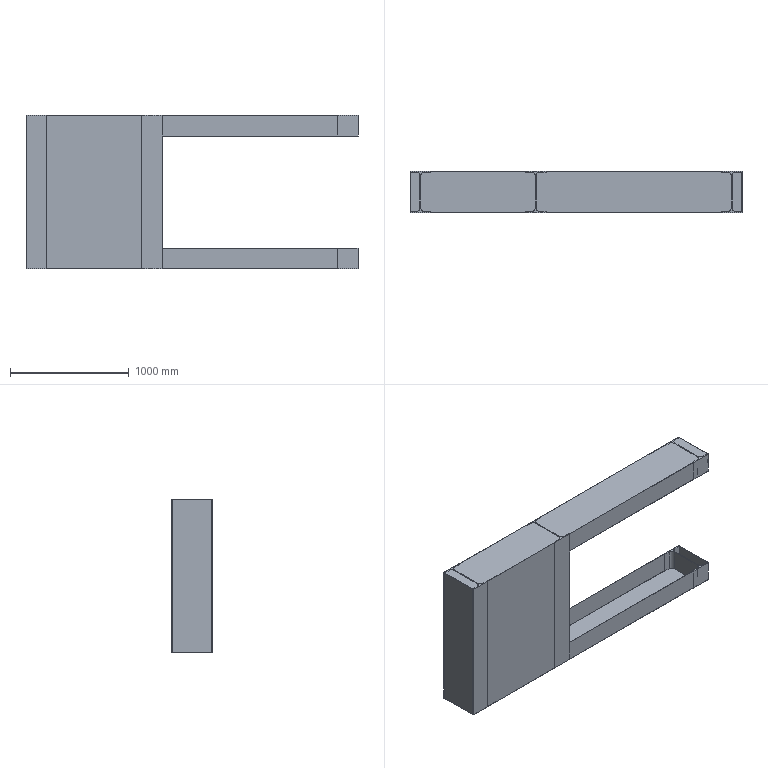Part | SolidWorks | features BaseBody 1 | 1 solid | 76 faces | box 2800 x 350 x 1296 mm | volume 23944279 mm3 | plane 60 | cylinder 16 | commonest cylinder face diameters 60 x16